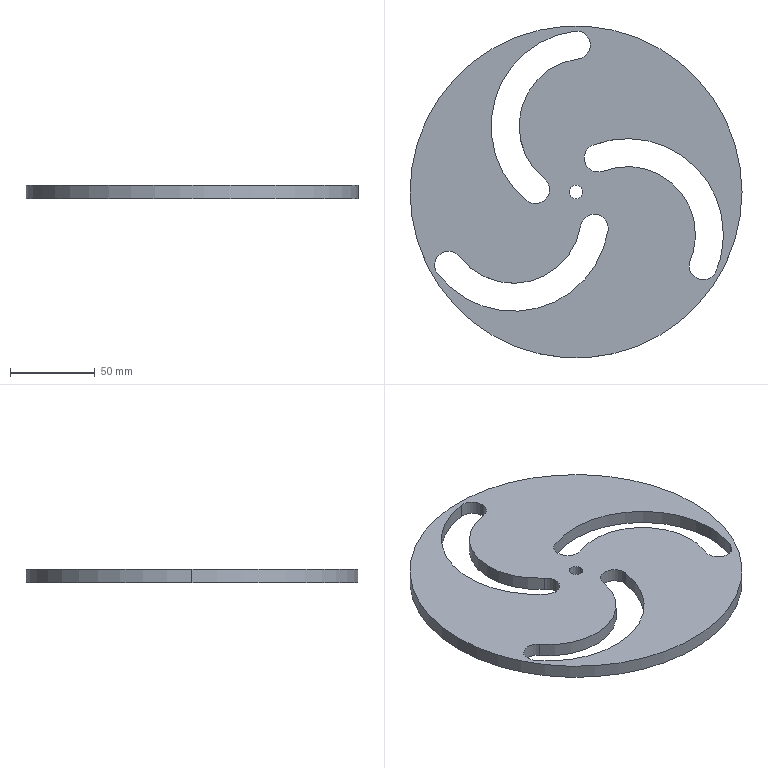Part | STEP file | Rotary disc | 1 solid | 23 faces | box 196 x 196 x 8 mm | volume 191240 mm3 | cylinder 21 | plane 2 | commonest cylinder face diameters 16.5 x9 80 x4 113 x4 8 x2 196 x2